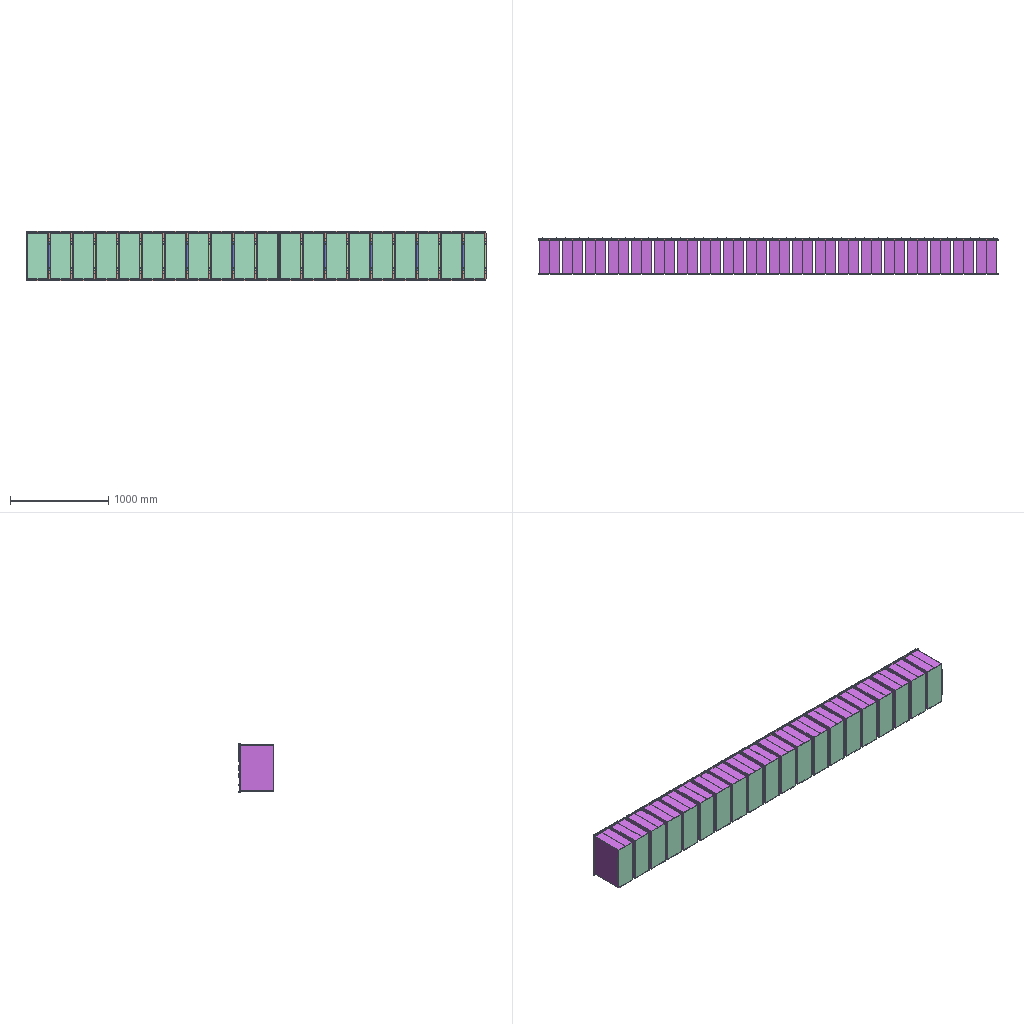Assembly | SolidWorks | 10 different items | 580 placed | box 4680 x 366 x 500 mm
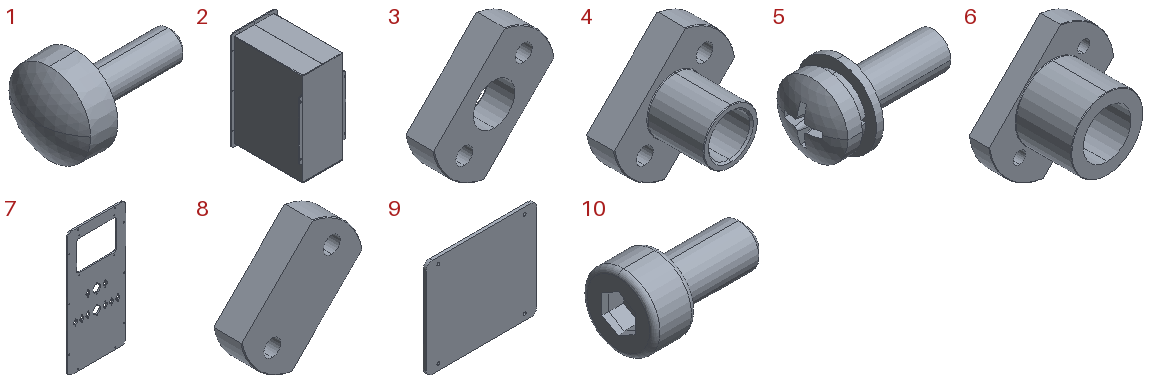Parts list (item | quantity | size | volume | features):
1 | x80 | 18 x 11 x 11 mm | 599.857 mm3 | features BaseBody 1
2 | x20 | 234 x 350 x 500 mm | 1268119 mm3 | features HoleWzd 4, ICE 4, 3DProfileFeature 3, Fillet 2, CosmeticWeldCutList 1, EdgeFlange 1, FlatPattern 1, SMBaseFlange 1, SheetMetal 1
3 | x20 | 34.452 x 8 x 34.452 mm | 3811 mm3 | features 3DProfileFeature 2, Chamfer 2, HoleWzd 2, ICE 2, Fillet 1, Revolution 1
4 | x20 | 34.452 x 24 x 34.452 mm | 5075 mm3 | features 3DProfileFeature 2, Chamfer 2, HoleWzd 2, Fillet 1, ICE 1, Revolution 1
5 | x200 | 14.964 x 9 x 9 mm | 319.965 mm3 | features BaseBody 3
6 | x20 | 49.497 x 30 x 49.497 mm | 16176 mm3 | features 3DProfileFeature 2, Chamfer 2, HoleWzd 2, ICE 1, Revolution 1
7 | x20 | 234 x 5 x 500 mm | 471230 mm3 | features 3DProfileFeature 5, HoleWzd 5, ICE 3, Fillet 2, Extrusion 1
8 | x20 | 34.452 x 8 x 34.452 mm | 4691 mm3 | features ICE 3, 3DProfileFeature 2, Chamfer 2, HoleWzd 2, Fillet 1, Revolution 1
9 | x20 | 180 x 5 x 160 mm | 143209 mm3 | features 3DProfileFeature 1, Extrusion 1, Fillet 1, HoleWzd 1
10 | x160 | 12 x 7 x 7 mm | 234.855 mm3 | features Chamfer 2, Fillet 1, ICE 1, Revolution 1
Mates (type | each side: item.copy, entity, surface, feature):
Coincident | 2.1 face plane Boss-Extrude2 | 7.1 face plane Boss-Extrude1
Concentric | 2.1 face cylinder M4 Tapped Hole2 | 7.1 face cylinder M4 Clearance Hole1 | 2 times
Coincident | 7.1 face plane Boss-Extrude1 | 3.1 face plane Revolve1
Concentric | 3.1 face cylinder Hole Size (% based on) Socket Head Cap Screw Type 1 | 7.1 face cylinder M4 Tapped Hole7 | 2 times
Coincident | 7.1 face plane Boss-Extrude1 | 8.1 face plane Revolve1
Concentric | 8.1 face cylinder Hole Size (% based on) Socket Head Cap Screw Type 1 | 7.1 face cylinder M4 Tapped Hole7 | 2 times
Coincident | 7.1 face plane Boss-Extrude1 | 6.1 face plane Revolve1
Coincident | 7.1 face plane Boss-Extrude1 | 4.1 face plane Revolve1
Concentric | 4.1 face cylinder G1/4 Tapped Hole1 | 7.1 face cylinder Cut-Extrude6
Concentric | 4.1 face cylinder Hole Size (% based on) Socket Head Cap Screw Type 1 | 7.1 face cylinder M4 Tapped Hole7
Coincident | 7.1 face plane Boss-Extrude1 | 9.1 face plane Boss-Extrude1
Concentric | 7.1 face cylinder M4 Tapped Hole4 | 9.1 face cylinder M4 Clearance Hole1 | 2 times
Concentric | 9.1 face cylinder M4 Clearance Hole1 | 1.1 face cylinder CRKB4_12
Concentric | 9.1 face cylinder M4 Clearance Hole1 | 1.2 face cylinder CRKB4_12
Concentric | 9.1 face cylinder M4 Clearance Hole1 | 1.3 face cylinder CRKB4_12
Concentric | 9.1 face cylinder M4 Clearance Hole1 | 1.4 face cylinder CRKB4_12
Coincident | 1.4 face plane CRKB4_12 | 1.3 face plane CRKB4_12
Coincident | 1.4 face plane CRKB4_12 | 1.1 face plane CRKB4_12
Coincident | 1.1 face plane CRKB4_12 | 1.2 face plane CRKB4_12
Coincident | 9.1 face plane Boss-Extrude1 | 1.1 face plane CRKB4_12
Concentric | 7.1 face cylinder M4 Clearance Hole1 | 5.1 face cylinder Screw M4×12 Stainless Steel GB 818-1-solid1
Coincident | 7.1 face plane Boss-Extrude1 | 5.1 edge
Concentric | 7.1 face cylinder M4 Clearance Hole1 | 5.2 face cylinder Screw M4×12 Stainless Steel GB 818-1-solid1
Concentric | 7.1 face cylinder M4 Clearance Hole1 | 5.3 face cylinder Screw M4×12 Stainless Steel GB 818-1-solid1
Concentric | 7.1 face cylinder M4 Clearance Hole1 | 5.4 face cylinder Screw M4×12 Stainless Steel GB 818-1-solid1
Concentric | 7.1 face cylinder M4 Clearance Hole1 | 5.5 face cylinder Screw M4×12 Stainless Steel GB 818-1-solid1
Concentric | 7.1 face cylinder M4 Clearance Hole1 | 5.6 face cylinder Screw M4×12 Stainless Steel GB 818-1-solid1
Concentric | 7.1 face cylinder M4 Clearance Hole1 | 5.7 face cylinder Screw M4×12 Stainless Steel GB 818-1-solid1
Concentric | 7.1 face cylinder M4 Clearance Hole1 | 5.8 face cylinder Screw M4×12 Stainless Steel GB 818-1-solid1
Concentric | 7.1 face cylinder M4 Clearance Hole1 | 5.9 face cylinder Screw M4×12 Stainless Steel GB 818-1-solid1
Concentric | 7.1 face cylinder M4 Clearance Hole1 | 5.10 face cylinder Screw M4×12 Stainless Steel GB 818-1-solid1
Coincident | 5.7 face plane B63000041  Flat Washer Grade A  ∅4 Stainless Steel 304  GB.T 97.1-2002-1-solid1 | 5.6 face plane B63000041  Flat Washer Grade A  ∅4 Stainless Steel 304  GB.T 97.1-2002-1-solid1
Coincident | 5.7 face plane B63000041  Flat Washer Grade A  ∅4 Stainless Steel 304  GB.T 97.1-2002-1-solid1 | 5.8 face plane B63000041  Flat Washer Grade A  ∅4 Stainless Steel 304  GB.T 97.1-2002-1-solid1
Coincident | 5.9 face plane B63000041  Flat Washer Grade A  ∅4 Stainless Steel 304  GB.T 97.1-2002-1-solid1 | 5.8 face plane B63000041  Flat Washer Grade A  ∅4 Stainless Steel 304  GB.T 97.1-2002-1-solid1
Coincident | 5.9 face plane B63000041  Flat Washer Grade A  ∅4 Stainless Steel 304  GB.T 97.1-2002-1-solid1 | 5.10 face plane B63000041  Flat Washer Grade A  ∅4 Stainless Steel 304  GB.T 97.1-2002-1-solid1
Coincident | 5.5 face plane B63000041  Flat Washer Grade A  ∅4 Stainless Steel 304  GB.T 97.1-2002-1-solid1 | 5.10 face plane B63000041  Flat Washer Grade A  ∅4 Stainless Steel 304  GB.T 97.1-2002-1-solid1
Coincident | 5.5 face plane B63000041  Flat Washer Grade A  ∅4 Stainless Steel 304  GB.T 97.1-2002-1-solid1 | 5.4 face plane B63000041  Flat Washer Grade A  ∅4 Stainless Steel 304  GB.T 97.1-2002-1-solid1
Coincident | 7.1 face plane Boss-Extrude1 | 5.3 face plane B63000041  Flat Washer Grade A  ∅4 Stainless Steel 304  GB.T 97.1-2002-1-solid1
Concentric | 8.1 face cylinder Hole Size (% based on) Socket Head Cap Screw Type 1 | 10.1 face cylinder Revolve1
Coincident | 8.1 face plane Hole Size (% based on) Socket Head Cap Screw Type 1 | 10.1 face plane Revolve1
Concentric | 8.1 face cylinder Hole Size (% based on) Socket Head Cap Screw Type 1 | 10.2 face cylinder Revolve1
Coincident | 8.1 face plane Hole Size (% based on) Socket Head Cap Screw Type 1 | 10.2 face plane Revolve1
Concentric | 3.1 face cylinder Hole Size (% based on) Socket Head Cap Screw Type 1 | 10.3 face cylinder Revolve1
Coincident | 3.1 face plane Hole Size (% based on) Socket Head Cap Screw Type 1 | 10.3 face plane Revolve1
Concentric | 3.1 face cylinder Hole Size (% based on) Socket Head Cap Screw Type 1 | 10.4 face cylinder Revolve1
Coincident | 3.1 face plane Hole Size (% based on) Socket Head Cap Screw Type 1 | 10.4 face plane Revolve1
Concentric | 4.1 face cylinder Hole Size (% based on) Socket Head Cap Screw Type 1 | 10.5 face cylinder Revolve1
Coincident | 4.1 face plane Hole Size (% based on) Socket Head Cap Screw Type 1 | 10.5 face plane Revolve1
Concentric | 4.1 face cylinder Hole Size (% based on) Socket Head Cap Screw Type 1 | 10.6 face cylinder Revolve1
Coincident | 4.1 face plane Hole Size (% based on) Socket Head Cap Screw Type 1 | 10.6 face plane Revolve1
Concentric | 6.1 face cylinder Hole Size (% based on) Socket Head Cap Screw Type 1 | 10.7 face cylinder Revolve1
Coincident | 6.1 face plane Hole Size (% based on) Socket Head Cap Screw Type 1 | 10.7 face plane Revolve1
Concentric | 6.1 face cylinder Hole Size (% based on) Socket Head Cap Screw Type 1 | 10.8 face cylinder Revolve1
Coincident | 6.1 face plane Hole Size (% based on) Socket Head Cap Screw Type 1 | 10.8 face plane Revolve1
Coincident | 5.1 face plane B63000041  Flat Washer Grade A  ∅4 Stainless Steel 304  GB.T 97.1-2002-1-solid1 | 5.2 face plane B63000041  Flat Washer Grade A  ∅4 Stainless Steel 304  GB.T 97.1-2002-1-solid1
Coincident | 5.2 face plane B63000041  Flat Washer Grade A  ∅4 Stainless Steel 304  GB.T 97.1-2002-1-solid1 | 5.4 face plane B63000041  Flat Washer Grade A  ∅4 Stainless Steel 304  GB.T 97.1-2002-1-solid1
Concentric | 7.1 face cylinder Cut-Extrude3 | 6.1 face cylinder Revolve1
Concentric | 7.1 face cylinder M4 Tapped Hole3 | 6.1 face cylinder Hole Size (% based on) Socket Head Cap Screw Type 1